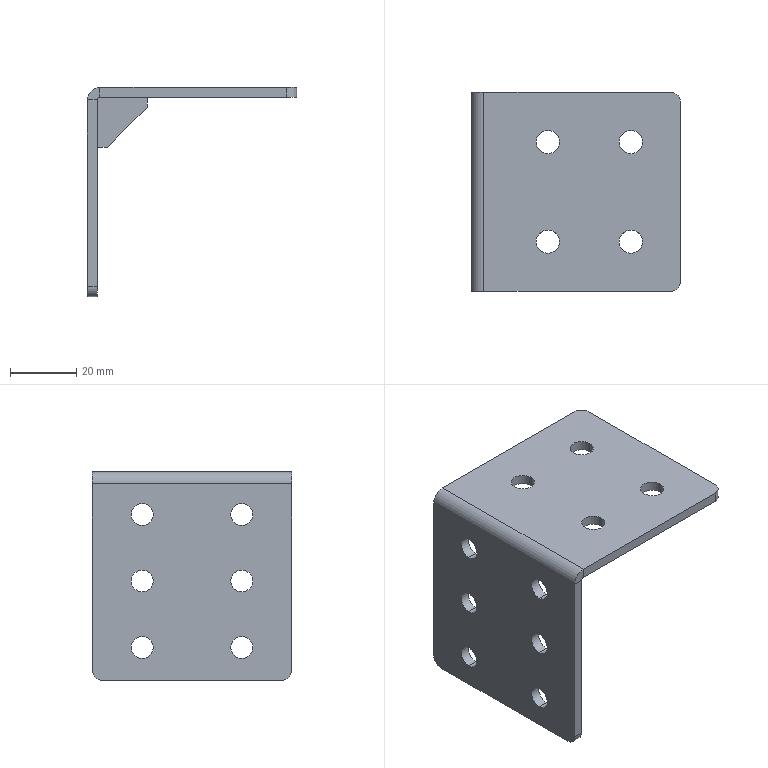Part | SolidWorks | features HoleWzd 2, Fillet 1, FlatPattern 1, ICE 1, SMBaseFlange 1, SheetMetal 1 | 1 solid | 44 faces | box 63 x 60 x 63 mm | volume 21324 mm3 | cylinder 27 | plane 17 | commonest cylinder face diameters 6.6 x12 7 x8 6 x4 1.5 x2 7.5 x1
STEP:
#1=CARTESIAN_POINT('',(23.5,45.,3.));
#2=VERTEX_POINT('',#1);
#3=CARTESIAN_POINT('',(16.5,45.,3.));
#4=VERTEX_POINT('',#3);
#5=CARTESIAN_POINT('',(20.,45.,3.));
#6=DIRECTION('',(0.,0.,-1.));
#7=DIRECTION('',(-1.,0.,0.));
#8=AXIS2_PLACEMENT_3D('',#5,#6,#7);
#9=CIRCLE('',#8,3.5);
#10=EDGE_CURVE('',#2,#4,#9,.T.);
#11=ORIENTED_EDGE('',*,*,#10,.F.);
#12=CARTESIAN_POINT('',(23.5,45.,0.));
#13=VERTEX_POINT('',#12);
#14=CARTESIAN_POINT('',(23.5,45.,0.));
#15=DIRECTION('',(0.,0.,-1.));
#16=VECTOR('',#15,1000.);
#17=LINE('',#14,#16);
#18=EDGE_CURVE('',#2,#13,#17,.T.);
#19=ORIENTED_EDGE('',*,*,#18,.T.);
#20=CARTESIAN_POINT('',(16.5,45.,0.));
#21=VERTEX_POINT('',#20);
#22=CARTESIAN_POINT('',(20.,45.,0.));
#23=DIRECTION('',(0.,0.,-1.));
#24=DIRECTION('',(-1.,0.,0.));
#25=AXIS2_PLACEMENT_3D('',#22,#23,#24);
#26=CIRCLE('',#25,3.5);
#27=EDGE_CURVE('',#13,#21,#26,.T.);
#28=ORIENTED_EDGE('',*,*,#27,.T.);
#29=CARTESIAN_POINT('',(16.5,45.,0.));
#30=DIRECTION('',(0.,0.,-1.));
#31=VECTOR('',#30,1000.);
#32=LINE('',#29,#31);
#33=EDGE_CURVE('',#4,#21,#32,.T.);
#34=ORIENTED_EDGE('',*,*,#33,.F.);
#35=EDGE_LOOP('',(#11,#19,#28,#34));
#36=FACE_OUTER_BOUND('',#35,.T.);
#37=CARTESIAN_POINT('',(20.,45.,0.));
#38=DIRECTION('',(0.,0.,-1.));
#39=DIRECTION('',(-1.,0.,0.));
#40=AXIS2_PLACEMENT_3D('',#37,#38,#39);
#41=CYLINDRICAL_SURFACE('',#40,3.5);
#42=ADVANCED_FACE('',(#36),#41,.F.);
#43=CARTESIAN_POINT('',(23.5,15.,3.));
#44=VERTEX_POINT('',#43);
#45=CARTESIAN_POINT('',(16.5,15.,3.));
#46=VERTEX_POINT('',#45);
#47=CARTESIAN_POINT('',(20.,15.,3.));
#48=DIRECTION('',(0.,0.,-1.));
#49=DIRECTION('',(-1.,0.,0.));
#50=AXIS2_PLACEMENT_3D('',#47,#48,#49);
#51=CIRCLE('',#50,3.5);
#52=EDGE_CURVE('',#44,#46,#51,.T.);
#53=ORIENTED_EDGE('',*,*,#52,.F.);
#54=CARTESIAN_POINT('',(23.5,15.,0.));
#55=VERTEX_POINT('',#54);
#56=CARTESIAN_POINT('',(23.5,15.,0.));
#57=DIRECTION('',(0.,0.,-1.));
#58=VECTOR('',#57,1000.);
#59=LINE('',#56,#58);
#60=EDGE_CURVE('',#44,#55,#59,.T.);
#61=ORIENTED_EDGE('',*,*,#60,.T.);
#62=CARTESIAN_POINT('',(16.5,15.,0.));
#63=VERTEX_POINT('',#62);
#64=CARTESIAN_POINT('',(20.,15.,0.));
#65=DIRECTION('',(0.,0.,-1.));
#66=DIRECTION('',(-1.,0.,0.));
#67=AXIS2_PLACEMENT_3D('',#64,#65,#66);
#68=CIRCLE('',#67,3.5);
#69=EDGE_CURVE('',#55,#63,#68,.T.);
#70=ORIENTED_EDGE('',*,*,#69,.T.);
#71=CARTESIAN_POINT('',(16.5,15.,0.));
#72=DIRECTION('',(0.,0.,-1.));
#73=VECTOR('',#72,1000.);
#74=LINE('',#71,#73);
#75=EDGE_CURVE('',#46,#63,#74,.T.);
#76=ORIENTED_EDGE('',*,*,#75,.F.);
#77=EDGE_LOOP('',(#53,#61,#70,#76));
#78=FACE_OUTER_BOUND('',#77,.T.);
#79=CARTESIAN_POINT('',(20.,15.,0.));
#80=DIRECTION('',(0.,0.,-1.));
#81=DIRECTION('',(-1.,0.,0.));
#82=AXIS2_PLACEMENT_3D('',#79,#80,#81);
#83=CYLINDRICAL_SURFACE('',#82,3.5);
#84=ADVANCED_FACE('',(#78),#83,.F.);
#85=CARTESIAN_POINT('',(48.5,45.,3.));
#86=VERTEX_POINT('',#85);
#87=CARTESIAN_POINT('',(41.5,45.,3.));
#88=VERTEX_POINT('',#87);
#89=CARTESIAN_POINT('',(45.,45.,3.));
#90=DIRECTION('',(0.,0.,-1.));
#91=DIRECTION('',(-1.,0.,0.));
#92=AXIS2_PLACEMENT_3D('',#89,#90,#91);
#93=CIRCLE('',#92,3.5);
#94=EDGE_CURVE('',#86,#88,#93,.T.);
#95=ORIENTED_EDGE('',*,*,#94,.F.);
#96=CARTESIAN_POINT('',(48.5,45.,0.));
#97=VERTEX_POINT('',#96);
#98=CARTESIAN_POINT('',(48.5,45.,0.));
#99=DIRECTION('',(0.,0.,-1.));
#100=VECTOR('',#99,1000.);
#101=LINE('',#98,#100);
#102=EDGE_CURVE('',#86,#97,#101,.T.);
#103=ORIENTED_EDGE('',*,*,#102,.T.);
#104=CARTESIAN_POINT('',(41.5,45.,0.));
#105=VERTEX_POINT('',#104);
#106=CARTESIAN_POINT('',(45.,45.,0.));
#107=DIRECTION('',(0.,0.,-1.));
#108=DIRECTION('',(-1.,0.,0.));
#109=AXIS2_PLACEMENT_3D('',#106,#107,#108);
#110=CIRCLE('',#109,3.5);
#111=EDGE_CURVE('',#97,#105,#110,.T.);
#112=ORIENTED_EDGE('',*,*,#111,.T.);
#113=CARTESIAN_POINT('',(41.5,45.,0.));
#114=DIRECTION('',(0.,0.,-1.));
#115=VECTOR('',#114,1000.);
#116=LINE('',#113,#115);
#117=EDGE_CURVE('',#88,#105,#116,.T.);
#118=ORIENTED_EDGE('',*,*,#117,.F.);
#119=EDGE_LOOP('',(#95,#103,#112,#118));
#120=FACE_OUTER_BOUND('',#119,.T.);
#121=CARTESIAN_POINT('',(45.,45.,0.));
#122=DIRECTION('',(0.,0.,-1.));
#123=DIRECTION('',(-1.,0.,0.));
#124=AXIS2_PLACEMENT_3D('',#121,#122,#123);
#125=CYLINDRICAL_SURFACE('',#124,3.5);
#126=ADVANCED_FACE('',(#120),#125,.F.);
#127=CARTESIAN_POINT('',(48.5,15.,3.));
#128=VERTEX_POINT('',#127);
#129=CARTESIAN_POINT('',(41.5,15.,3.));
#130=VERTEX_POINT('',#129);
#131=CARTESIAN_POINT('',(45.,15.,3.));
#132=DIRECTION('',(0.,0.,-1.));
#133=DIRECTION('',(-1.,0.,0.));
#134=AXIS2_PLACEMENT_3D('',#131,#132,#133);
#135=CIRCLE('',#134,3.5);
#136=EDGE_CURVE('',#128,#130,#135,.T.);
#137=ORIENTED_EDGE('',*,*,#136,.F.);
#138=CARTESIAN_POINT('',(48.5,15.,0.));
#139=VERTEX_POINT('',#138);
#140=CARTESIAN_POINT('',(48.5,15.,0.));
#141=DIRECTION('',(0.,0.,-1.));
#142=VECTOR('',#141,1000.);
#143=LINE('',#140,#142);
#144=EDGE_CURVE('',#128,#139,#143,.T.);
#145=ORIENTED_EDGE('',*,*,#144,.T.);
#146=CARTESIAN_POINT('',(41.5,15.,0.));
#147=VERTEX_POINT('',#146);
#148=CARTESIAN_POINT('',(45.,15.,0.));
#149=DIRECTION('',(0.,0.,-1.));
#150=DIRECTION('',(-1.,0.,0.));
#151=AXIS2_PLACEMENT_3D('',#148,#149,#150);
#152=CIRCLE('',#151,3.5);
#153=EDGE_CURVE('',#139,#147,#152,.T.);
#154=ORIENTED_EDGE('',*,*,#153,.T.);
#155=CARTESIAN_POINT('',(41.5,15.,0.));
#156=DIRECTION('',(0.,0.,-1.));
#157=VECTOR('',#156,1000.);
#158=LINE('',#155,#157);
#159=EDGE_CURVE('',#130,#147,#158,.T.);
#160=ORIENTED_EDGE('',*,*,#159,.F.);
#161=EDGE_LOOP('',(#137,#145,#154,#160));
#162=FACE_OUTER_BOUND('',#161,.T.);
#163=CARTESIAN_POINT('',(45.,15.,0.));
#164=DIRECTION('',(0.,0.,-1.));
#165=DIRECTION('',(-1.,0.,0.));
#166=AXIS2_PLACEMENT_3D('',#163,#164,#165);
#167=CYLINDRICAL_SURFACE('',#166,3.5);
#168=ADVANCED_FACE('',(#162),#167,.F.);
#169=CARTESIAN_POINT('',(-3.,45.,-46.7));
#170=VERTEX_POINT('',#169);
#171=CARTESIAN_POINT('',(-3.,45.,-53.3));
#172=VERTEX_POINT('',#171);
#173=CARTESIAN_POINT('',(-3.,45.,-50.));
#174=DIRECTION('',(1.,0.,0.));
#175=DIRECTION('',(0.,0.,-1.));
#176=AXIS2_PLACEMENT_3D('',#173,#174,#175);
#177=CIRCLE('',#176,3.3);
#178=EDGE_CURVE('',#170,#172,#177,.T.);
#179=ORIENTED_EDGE('',*,*,#178,.F.);
#180=CARTESIAN_POINT('',(0.,45.,-46.7));
#181=VERTEX_POINT('',#180);
#182=CARTESIAN_POINT('',(0.,45.,-46.7));
#183=DIRECTION('',(1.,0.,0.));
#184=VECTOR('',#183,1000.);
#185=LINE('',#182,#184);
#186=EDGE_CURVE('',#170,#181,#185,.T.);
#187=ORIENTED_EDGE('',*,*,#186,.T.);
#188=CARTESIAN_POINT('',(0.,45.,-53.3));
#189=VERTEX_POINT('',#188);
#190=CARTESIAN_POINT('',(0.,45.,-50.));
#191=DIRECTION('',(1.,0.,0.));
#192=DIRECTION('',(0.,0.,-1.));
#193=AXIS2_PLACEMENT_3D('',#190,#191,#192);
#194=CIRCLE('',#193,3.3);
#195=EDGE_CURVE('',#181,#189,#194,.T.);
#196=ORIENTED_EDGE('',*,*,#195,.T.);
#197=CARTESIAN_POINT('',(0.,45.,-53.3));
#198=DIRECTION('',(1.,0.,0.));
#199=VECTOR('',#198,1000.);
#200=LINE('',#197,#199);
#201=EDGE_CURVE('',#172,#189,#200,.T.);
#202=ORIENTED_EDGE('',*,*,#201,.F.);
#203=EDGE_LOOP('',(#179,#187,#196,#202));
#204=FACE_OUTER_BOUND('',#203,.T.);
#205=CARTESIAN_POINT('',(0.,45.,-50.));
#206=DIRECTION('',(1.,0.,0.));
#207=DIRECTION('',(0.,0.,-1.));
#208=AXIS2_PLACEMENT_3D('',#205,#206,#207);
#209=CYLINDRICAL_SURFACE('',#208,3.3);
#210=ADVANCED_FACE('',(#204),#209,.F.);
#211=CARTESIAN_POINT('',(-3.,45.,-26.7));
#212=VERTEX_POINT('',#211);
#213=CARTESIAN_POINT('',(-3.,45.,-33.3));
#214=VERTEX_POINT('',#213);
#215=CARTESIAN_POINT('',(-3.,45.,-30.));
#216=DIRECTION('',(1.,0.,0.));
#217=DIRECTION('',(0.,0.,-1.));
#218=AXIS2_PLACEMENT_3D('',#215,#216,#217);
#219=CIRCLE('',#218,3.3);
#220=EDGE_CURVE('',#212,#214,#219,.T.);
#221=ORIENTED_EDGE('',*,*,#220,.F.);
#222=CARTESIAN_POINT('',(0.,45.,-26.7));
#223=VERTEX_POINT('',#222);
#224=CARTESIAN_POINT('',(0.,45.,-26.7));
#225=DIRECTION('',(1.,0.,0.));
#226=VECTOR('',#225,1000.);
#227=LINE('',#224,#226);
#228=EDGE_CURVE('',#212,#223,#227,.T.);
#229=ORIENTED_EDGE('',*,*,#228,.T.);
#230=CARTESIAN_POINT('',(0.,45.,-33.3));
#231=VERTEX_POINT('',#230);
#232=CARTESIAN_POINT('',(0.,45.,-30.));
#233=DIRECTION('',(1.,0.,0.));
#234=DIRECTION('',(0.,0.,-1.));
#235=AXIS2_PLACEMENT_3D('',#232,#233,#234);
#236=CIRCLE('',#235,3.3);
#237=EDGE_CURVE('',#223,#231,#236,.T.);
#238=ORIENTED_EDGE('',*,*,#237,.T.);
#239=CARTESIAN_POINT('',(0.,45.,-33.3));
#240=DIRECTION('',(1.,0.,0.));
#241=VECTOR('',#240,1000.);
#242=LINE('',#239,#241);
#243=EDGE_CURVE('',#214,#231,#242,.T.);
#244=ORIENTED_EDGE('',*,*,#243,.F.);
#245=EDGE_LOOP('',(#221,#229,#238,#244));
#246=FACE_OUTER_BOUND('',#245,.T.);
#247=CARTESIAN_POINT('',(0.,45.,-30.));
#248=DIRECTION('',(1.,0.,0.));
#249=DIRECTION('',(0.,0.,-1.));
#250=AXIS2_PLACEMENT_3D('',#247,#248,#249);
#251=CYLINDRICAL_SURFACE('',#250,3.3);
#252=ADVANCED_FACE('',(#246),#251,.F.);
#253=CARTESIAN_POINT('',(-3.,45.,-6.7));
#254=VERTEX_POINT('',#253);
#255=CARTESIAN_POINT('',(-3.,45.,-13.3));
#256=VERTEX_POINT('',#255);
#257=CARTESIAN_POINT('',(-3.,45.,-10.));
#258=DIRECTION('',(1.,0.,0.));
#259=DIRECTION('',(0.,0.,-1.));
#260=AXIS2_PLACEMENT_3D('',#257,#258,#259);
#261=CIRCLE('',#260,3.3);
#262=EDGE_CURVE('',#254,#256,#261,.T.);
#263=ORIENTED_EDGE('',*,*,#262,.F.);
#264=CARTESIAN_POINT('',(0.,45.,-6.7));
#265=VERTEX_POINT('',#264);
#266=CARTESIAN_POINT('',(0.,45.,-6.7));
#267=DIRECTION('',(1.,0.,0.));
#268=VECTOR('',#267,1000.);
#269=LINE('',#266,#268);
#270=EDGE_CURVE('',#254,#265,#269,.T.);
#271=ORIENTED_EDGE('',*,*,#270,.T.);
#272=CARTESIAN_POINT('',(0.,45.,-13.3));
#273=VERTEX_POINT('',#272);
#274=CARTESIAN_POINT('',(0.,45.,-10.));
#275=DIRECTION('',(1.,0.,0.));
#276=DIRECTION('',(0.,0.,-1.));
#277=AXIS2_PLACEMENT_3D('',#274,#275,#276);
#278=CIRCLE('',#277,3.3);
#279=EDGE_CURVE('',#265,#273,#278,.T.);
#280=ORIENTED_EDGE('',*,*,#279,.T.);
#281=CARTESIAN_POINT('',(0.,45.,-13.3));
#282=DIRECTION('',(1.,0.,0.));
#283=VECTOR('',#282,1000.);
#284=LINE('',#281,#283);
#285=EDGE_CURVE('',#256,#273,#284,.T.);
#286=ORIENTED_EDGE('',*,*,#285,.F.);
#287=EDGE_LOOP('',(#263,#271,#280,#286));
#288=FACE_OUTER_BOUND('',#287,.T.);
#289=CARTESIAN_POINT('',(0.,45.,-10.));
#290=DIRECTION('',(1.,0.,0.));
#291=DIRECTION('',(0.,0.,-1.));
#292=AXIS2_PLACEMENT_3D('',#289,#290,#291);
#293=CYLINDRICAL_SURFACE('',#292,3.3);
#294=ADVANCED_FACE('',(#288),#293,.F.);
#295=CARTESIAN_POINT('',(-3.,15.,-46.7));
#296=VERTEX_POINT('',#295);
#297=CARTESIAN_POINT('',(-3.,15.,-53.3));
#298=VERTEX_POINT('',#297);
#299=CARTESIAN_POINT('',(-3.,15.,-50.));
#300=DIRECTION('',(1.,0.,0.));
#301=DIRECTION('',(0.,0.,-1.));
#302=AXIS2_PLACEMENT_3D('',#299,#300,#301);
#303=CIRCLE('',#302,3.3);
#304=EDGE_CURVE('',#296,#298,#303,.T.);
#305=ORIENTED_EDGE('',*,*,#304,.F.);
#306=CARTESIAN_POINT('',(0.,15.,-46.7));
#307=VERTEX_POINT('',#306);
#308=CARTESIAN_POINT('',(0.,15.,-46.7));
#309=DIRECTION('',(1.,0.,0.));
#310=VECTOR('',#309,1000.);
#311=LINE('',#308,#310);
#312=EDGE_CURVE('',#296,#307,#311,.T.);
#313=ORIENTED_EDGE('',*,*,#312,.T.);
#314=CARTESIAN_POINT('',(0.,15.,-53.3));
#315=VERTEX_POINT('',#314);
#316=CARTESIAN_POINT('',(0.,15.,-50.));
#317=DIRECTION('',(1.,0.,0.));
#318=DIRECTION('',(0.,0.,-1.));
#319=AXIS2_PLACEMENT_3D('',#316,#317,#318);
#320=CIRCLE('',#319,3.3);
#321=EDGE_CURVE('',#307,#315,#320,.T.);
#322=ORIENTED_EDGE('',*,*,#321,.T.);
#323=CARTESIAN_POINT('',(0.,15.,-53.3));
#324=DIRECTION('',(1.,0.,0.));
#325=VECTOR('',#324,1000.);
#326=LINE('',#323,#325);
#327=EDGE_CURVE('',#298,#315,#326,.T.);
#328=ORIENTED_EDGE('',*,*,#327,.F.);
#329=EDGE_LOOP('',(#305,#313,#322,#328));
#330=FACE_OUTER_BOUND('',#329,.T.);
#331=CARTESIAN_POINT('',(0.,15.,-50.));
#332=DIRECTION('',(1.,0.,0.));
#333=DIRECTION('',(0.,0.,-1.));
#334=AXIS2_PLACEMENT_3D('',#331,#332,#333);
#335=CYLINDRICAL_SURFACE('',#334,3.3);
#336=ADVANCED_FACE('',(#330),#335,.F.);
#337=CARTESIAN_POINT('',(-3.,15.,-26.7));
#338=VERTEX_POINT('',#337);
#339=CARTESIAN_POINT('',(-3.,15.,-33.3));
#340=VERTEX_POINT('',#339);
#341=CARTESIAN_POINT('',(-3.,15.,-30.));
#342=DIRECTION('',(1.,0.,0.));
#343=DIRECTION('',(0.,0.,-1.));
#344=AXIS2_PLACEMENT_3D('',#341,#342,#343);
#345=CIRCLE('',#344,3.3);
#346=EDGE_CURVE('',#338,#340,#345,.T.);
#347=ORIENTED_EDGE('',*,*,#346,.F.);
#348=CARTESIAN_POINT('',(0.,15.,-26.7));
#349=VERTEX_POINT('',#348);
#350=CARTESIAN_POINT('',(0.,15.,-26.7));
#351=DIRECTION('',(1.,0.,0.));
#352=VECTOR('',#351,1000.);
#353=LINE('',#350,#352);
#354=EDGE_CURVE('',#338,#349,#353,.T.);
#355=ORIENTED_EDGE('',*,*,#354,.T.);
#356=CARTESIAN_POINT('',(0.,15.,-33.3));
#357=VERTEX_POINT('',#356);
#358=CARTESIAN_POINT('',(0.,15.,-30.));
#359=DIRECTION('',(1.,0.,0.));
#360=DIRECTION('',(0.,0.,-1.));
#361=AXIS2_PLACEMENT_3D('',#358,#359,#360);
#362=CIRCLE('',#361,3.3);
#363=EDGE_CURVE('',#349,#357,#362,.T.);
#364=ORIENTED_EDGE('',*,*,#363,.T.);
#365=CARTESIAN_POINT('',(0.,15.,-33.3));
#366=DIRECTION('',(1.,0.,0.));
#367=VECTOR('',#366,1000.);
#368=LINE('',#365,#367);
#369=EDGE_CURVE('',#340,#357,#368,.T.);
#370=ORIENTED_EDGE('',*,*,#369,.F.);
#371=EDGE_LOOP('',(#347,#355,#364,#370));
#372=FACE_OUTER_BOUND('',#371,.T.);
#373=CARTESIAN_POINT('',(0.,15.,-30.));
#374=DIRECTION('',(1.,0.,0.));
#375=DIRECTION('',(0.,0.,-1.));
#376=AXIS2_PLACEMENT_3D('',#373,#374,#375);
#377=CYLINDRICAL_SURFACE('',#376,3.3);
#378=ADVANCED_FACE('',(#372),#377,.F.);
#379=CARTESIAN_POINT('',(-3.,15.,-6.7));
#380=VERTEX_POINT('',#379);
#381=CARTESIAN_POINT('',(-3.,15.,-13.3));
#382=VERTEX_POINT('',#381);
#383=CARTESIAN_POINT('',(-3.,15.,-10.));
#384=DIRECTION('',(1.,0.,0.));
#385=DIRECTION('',(0.,0.,-1.));
#386=AXIS2_PLACEMENT_3D('',#383,#384,#385);
#387=CIRCLE('',#386,3.3);
#388=EDGE_CURVE('',#380,#382,#387,.T.);
#389=ORIENTED_EDGE('',*,*,#388,.F.);
#390=CARTESIAN_POINT('',(0.,15.,-6.7));
#391=VERTEX_POINT('',#390);
#392=CARTESIAN_POINT('',(0.,15.,-6.7));
#393=DIRECTION('',(1.,0.,0.));
#394=VECTOR('',#393,1000.);
#395=LINE('',#392,#394);
#396=EDGE_CURVE('',#380,#391,#395,.T.);
#397=ORIENTED_EDGE('',*,*,#396,.T.);
#398=CARTESIAN_POINT('',(0.,15.,-13.3));
#399=VERTEX_POINT('',#398);
#400=CARTESIAN_POINT('',(0.,15.,-10.));
#401=DIRECTION('',(1.,0.,0.));
#402=DIRECTION('',(0.,0.,-1.));
#403=AXIS2_PLACEMENT_3D('',#400,#401,#402);
#404=CIRCLE('',#403,3.3);
#405=EDGE_CURVE('',#391,#399,#404,.T.);
#406=ORIENTED_EDGE('',*,*,#405,.T.);
#407=CARTESIAN_POINT('',(0.,15.,-13.3));
#408=DIRECTION('',(1.,0.,0.));
#409=VECTOR('',#408,1000.);
#410=LINE('',#407,#409);
#411=EDGE_CURVE('',#382,#399,#410,.T.);
#412=ORIENTED_EDGE('',*,*,#411,.F.);
#413=EDGE_LOOP('',(#389,#397,#406,#412));
#414=FACE_OUTER_BOUND('',#413,.T.);
#415=CARTESIAN_POINT('',(0.,15.,-10.));
#416=DIRECTION('',(1.,0.,0.));
#417=DIRECTION('',(0.,0.,-1.));
#418=AXIS2_PLACEMENT_3D('',#415,#416,#417);
#419=CYLINDRICAL_SURFACE('',#418,3.3);
#420=ADVANCED_FACE('',(#414),#419,.F.);
#421=CARTESIAN_POINT('',(0.,28.5,-0.75));
#422=VERTEX_POINT('',#421);
#423=CARTESIAN_POINT('',(0.,0.,-0.75));
#424=VERTEX_POINT('',#423);
#425=CARTESIAN_POINT('',(0.,60.,-0.75));
#426=DIRECTION('',(0.,-1.,0.));
#427=VECTOR('',#426,1000.);
#428=LINE('',#425,#427);
#429=EDGE_CURVE('',#422,#424,#428,.T.);
#430=ORIENTED_EDGE('',*,*,#429,.F.);
#431=CARTESIAN_POINT('',(0.75,28.5,0.));
#432=VERTEX_POINT('',#431);
#433=CARTESIAN_POINT('',(0.75,28.5,-0.75));
#434=DIRECTION('',(0.,1.,0.));
#435=DIRECTION('',(0.,0.,1.));
#436=AXIS2_PLACEMENT_3D('',#433,#434,#435);
#437=CIRCLE('',#436,0.75);
#438=EDGE_CURVE('',#422,#432,#437,.T.);
#439=ORIENTED_EDGE('',*,*,#438,.T.);
#440=CARTESIAN_POINT('',(0.75,0.,0.));
#441=VERTEX_POINT('',#440);
#442=CARTESIAN_POINT('',(0.75,60.,0.));
#443=DIRECTION('',(0.,-1.,0.));
#444=VECTOR('',#443,1000.);
#445=LINE('',#442,#444);
#446=EDGE_CURVE('',#432,#441,#445,.T.);
#447=ORIENTED_EDGE('',*,*,#446,.T.);
#448=CARTESIAN_POINT('',(0.75,0.,-0.75));
#449=DIRECTION('',(0.,1.,0.));
#450=DIRECTION('',(0.,0.,-1.));
#451=AXIS2_PLACEMENT_3D('',#448,#449,#450);
#452=CIRCLE('',#451,0.75);
#453=EDGE_CURVE('',#424,#441,#452,.T.);
#454=ORIENTED_EDGE('',*,*,#453,.F.);
#455=EDGE_LOOP('',(#430,#439,#447,#454));
#456=FACE_OUTER_BOUND('',#455,.T.);
#457=CARTESIAN_POINT('',(0.75,60.,-0.75));
#458=DIRECTION('',(0.,-1.,0.));
#459=DIRECTION('',(0.,0.,-1.));
#460=AXIS2_PLACEMENT_3D('',#457,#458,#459);
#461=CYLINDRICAL_SURFACE('',#460,0.75);
#462=ADVANCED_FACE('',(#456),#461,.F.);
#463=CARTESIAN_POINT('',(0.75,60.,0.));
#464=VERTEX_POINT('',#463);
#465=CARTESIAN_POINT('',(0.75,60.,3.));
#466=VERTEX_POINT('',#465);
#467=CARTESIAN_POINT('',(0.75,60.,0.));
#468=DIRECTION('',(0.,0.,1.));
#469=VECTOR('',#468,1000.);
#470=LINE('',#467,#469);
#471=EDGE_CURVE('',#464,#466,#470,.T.);
#472=ORIENTED_EDGE('',*,*,#471,.F.);
#473=CARTESIAN_POINT('',(0.,60.,-0.75));
#474=VERTEX_POINT('',#473);
#475=CARTESIAN_POINT('',(0.75,60.,-0.75));
#476=DIRECTION('',(0.,1.,0.));
#477=DIRECTION('',(0.,0.,-1.));
#478=AXIS2_PLACEMENT_3D('',#475,#476,#477);
#479=CIRCLE('',#478,0.75);
#480=EDGE_CURVE('',#474,#464,#479,.T.);
#481=ORIENTED_EDGE('',*,*,#480,.F.);
#482=CARTESIAN_POINT('',(-3.,60.,-0.75));
#483=VERTEX_POINT('',#482);
#484=CARTESIAN_POINT('',(-3.,60.,-0.75));
#485=DIRECTION('',(1.,0.,0.));
#486=VECTOR('',#485,1000.);
#487=LINE('',#484,#486);
#488=EDGE_CURVE('',#483,#474,#487,.T.);
#489=ORIENTED_EDGE('',*,*,#488,.F.);
#490=CARTESIAN_POINT('',(0.75,60.,-0.75));
#491=DIRECTION('',(0.,1.,0.));
#492=DIRECTION('',(1.,0.,0.));
#493=AXIS2_PLACEMENT_3D('',#490,#491,#492);
#494=CIRCLE('',#493,3.75);
#495=EDGE_CURVE('',#483,#466,#494,.T.);
#496=ORIENTED_EDGE('',*,*,#495,.T.);
#497=EDGE_LOOP('',(#472,#481,#489,#496));
#498=FACE_OUTER_BOUND('',#497,.T.);
#499=CARTESIAN_POINT('',(0.75,60.,0.));
#500=DIRECTION('',(0.,1.,0.));
#501=DIRECTION('',(0.,0.,1.));
#502=AXIS2_PLACEMENT_3D('',#499,#500,#501);
#503=PLANE('',#502);
#504=ADVANCED_FACE('',(#498),#503,.T.);
#505=CARTESIAN_POINT('',(57.,60.,3.));
#506=VERTEX_POINT('',#505);
#507=CARTESIAN_POINT('',(0.,60.,3.));
#508=DIRECTION('',(1.,0.,0.));
#509=VECTOR('',#508,1000.);
#510=LINE('',#507,#509);
#511=EDGE_CURVE('',#466,#506,#510,.T.);
#512=ORIENTED_EDGE('',*,*,#511,.T.);
#513=CARTESIAN_POINT('',(57.,60.,0.));
#514=VERTEX_POINT('',#513);
#515=CARTESIAN_POINT('',(57.,60.,-0.75));
#516=DIRECTION('',(0.,0.,-1.));
#517=VECTOR('',#516,1000.);
#518=LINE('',#515,#517);
#519=EDGE_CURVE('',#506,#514,#518,.T.);
#520=ORIENTED_EDGE('',*,*,#519,.T.);
#521=CARTESIAN_POINT('',(0.,60.,0.));
#522=DIRECTION('',(1.,0.,0.));
#523=VECTOR('',#522,1000.);
#524=LINE('',#521,#523);
#525=EDGE_CURVE('',#464,#514,#524,.T.);
#526=ORIENTED_EDGE('',*,*,#525,.F.);
#527=ORIENTED_EDGE('',*,*,#471,.T.);
#528=EDGE_LOOP('',(#512,#520,#526,#527));
#529=FACE_OUTER_BOUND('',#528,.T.);
#530=CARTESIAN_POINT('',(-3.,60.,-0.75));
#531=DIRECTION('',(0.,1.,0.));
#532=DIRECTION('',(0.,0.,1.));
#533=AXIS2_PLACEMENT_3D('',#530,#531,#532);
#534=PLANE('',#533);
#535=ADVANCED_FACE('',(#529),#534,.T.);
#536=CARTESIAN_POINT('',(-3.,0.,-0.75));
#537=VERTEX_POINT('',#536);
#538=CARTESIAN_POINT('',(0.,0.,-0.75));
#539=DIRECTION('',(-1.,0.,0.));
#540=VECTOR('',#539,1000.);
#541=LINE('',#538,#540);
#542=EDGE_CURVE('',#424,#537,#541,.T.);
#543=ORIENTED_EDGE('',*,*,#542,.F.);
#544=ORIENTED_EDGE('',*,*,#453,.T.);
#545=CARTESIAN_POINT('',(0.75,0.,3.));
#546=VERTEX_POINT('',#545);
#547=CARTESIAN_POINT('',(0.75,0.,3.));
#548=DIRECTION('',(0.,0.,-1.));
#549=VECTOR('',#548,1000.);
#550=LINE('',#547,#549);
#551=EDGE_CURVE('',#546,#441,#550,.T.);
#552=ORIENTED_EDGE('',*,*,#551,.F.);
#553=CARTESIAN_POINT('',(0.75,0.,-0.75));
#554=DIRECTION('',(0.,1.,0.));
#555=DIRECTION('',(1.,0.,0.));
#556=AXIS2_PLACEMENT_3D('',#553,#554,#555);
#557=CIRCLE('',#556,3.75);
#558=EDGE_CURVE('',#537,#546,#557,.T.);
#559=ORIENTED_EDGE('',*,*,#558,.F.);
#560=EDGE_LOOP('',(#543,#544,#552,#559));
#561=FACE_OUTER_BOUND('',#560,.T.);
#562=CARTESIAN_POINT('',(0.,0.,-0.75));
#563=DIRECTION('',(0.,-1.,0.));
#564=DIRECTION('',(0.,0.,-1.));
#565=AXIS2_PLACEMENT_3D('',#562,#563,#564);
#566=PLANE('',#565);
#567=ADVANCED_FACE('',(#561),#566,.T.);
#568=CARTESIAN_POINT('',(-3.,0.,-57.));
#569=VERTEX_POINT('',#568);
#570=CARTESIAN_POINT('',(-3.,0.,-60.));
#571=DIRECTION('',(0.,0.,1.));
#572=VECTOR('',#571,1000.);
#573=LINE('',#570,#572);
#574=EDGE_CURVE('',#569,#537,#573,.T.);
#575=ORIENTED_EDGE('',*,*,#574,.F.);
#576=CARTESIAN_POINT('',(0.,0.,-57.));
#577=VERTEX_POINT('',#576);
#578=CARTESIAN_POINT('',(0.75,0.,-57.));
#579=DIRECTION('',(1.,0.,0.));
#580=VECTOR('',#579,1000.);
#581=LINE('',#578,#580);
#582=EDGE_CURVE('',#569,#577,#581,.T.);
#583=ORIENTED_EDGE('',*,*,#582,.T.);
#584=CARTESIAN_POINT('',(0.,0.,-60.));
#585=DIRECTION('',(0.,0.,1.));
#586=VECTOR('',#585,1000.);
#587=LINE('',#584,#586);
#588=EDGE_CURVE('',#577,#424,#587,.T.);
#589=ORIENTED_EDGE('',*,*,#588,.T.);
#590=ORIENTED_EDGE('',*,*,#542,.T.);
#591=EDGE_LOOP('',(#575,#583,#589,#590));
#592=FACE_OUTER_BOUND('',#591,.T.);
#593=CARTESIAN_POINT('',(0.75,0.,3.));
#594=DIRECTION('',(0.,-1.,0.));
#595=DIRECTION('',(0.,0.,-1.));
#596=AXIS2_PLACEMENT_3D('',#593,#594,#595);
#597=PLANE('',#596);
#598=ADVANCED_FACE('',(#592),#597,.T.);
#599=CARTESIAN_POINT('',(20.,45.,3.));
#600=DIRECTION('',(0.,0.,-1.));
#601=DIRECTION('',(-1.,0.,0.));
#602=AXIS2_PLACEMENT_3D('',#599,#600,#601);
#603=CIRCLE('',#602,3.5);
#604=EDGE_CURVE('',#4,#2,#603,.T.);
#605=ORIENTED_EDGE('',*,*,#604,.T.);
#606=ORIENTED_EDGE('',*,*,#10,.T.);
#607=EDGE_LOOP('',(#605,#606));
#608=FACE_BOUND('',#607,.T.);
#609=CARTESIAN_POINT('',(20.,15.,3.));
#610=DIRECTION('',(0.,0.,-1.));
#611=DIRECTION('',(-1.,0.,0.));
#612=AXIS2_PLACEMENT_3D('',#609,#610,#611);
#613=CIRCLE('',#612,3.5);
#614=EDGE_CURVE('',#46,#44,#613,.T.);
#615=ORIENTED_EDGE('',*,*,#614,.T.);
#616=ORIENTED_EDGE('',*,*,#52,.T.);
#617=EDGE_LOOP('',(#615,#616));
#618=FACE_BOUND('',#617,.T.);
#619=CARTESIAN_POINT('',(45.,45.,3.));
#620=DIRECTION('',(0.,0.,-1.));
#621=DIRECTION('',(-1.,0.,0.));
#622=AXIS2_PLACEMENT_3D('',#619,#620,#621);
#623=CIRCLE('',#622,3.5);
#624=EDGE_CURVE('',#88,#86,#623,.T.);
#625=ORIENTED_EDGE('',*,*,#624,.T.);
#626=ORIENTED_EDGE('',*,*,#94,.T.);
#627=EDGE_LOOP('',(#625,#626));
#628=FACE_BOUND('',#627,.T.);
#629=CARTESIAN_POINT('',(45.,15.,3.));
#630=DIRECTION('',(0.,0.,-1.));
#631=DIRECTION('',(-1.,0.,0.));
#632=AXIS2_PLACEMENT_3D('',#629,#630,#631);
#633=CIRCLE('',#632,3.5);
#634=EDGE_CURVE('',#130,#128,#633,.T.);
#635=ORIENTED_EDGE('',*,*,#634,.T.);
#636=ORIENTED_EDGE('',*,*,#136,.T.);
#637=EDGE_LOOP('',(#635,#636));
#638=FACE_BOUND('',#637,.T.);
#639=CARTESIAN_POINT('',(57.,0.,3.));
#640=VERTEX_POINT('',#639);
#641=CARTESIAN_POINT('',(0.,0.,3.));
#642=DIRECTION('',(1.,0.,0.));
#643=VECTOR('',#642,1000.);
#644=LINE('',#641,#643);
#645=EDGE_CURVE('',#546,#640,#644,.T.);
#646=ORIENTED_EDGE('',*,*,#645,.T.);
#647=CARTESIAN_POINT('',(60.,3.,3.));
#648=VERTEX_POINT('',#647);
#649=CARTESIAN_POINT('',(57.,3.,3.));
#650=DIRECTION('',(0.,0.,1.));
#651=DIRECTION('',(-1.,0.,0.));
#652=AXIS2_PLACEMENT_3D('',#649,#650,#651);
#653=CIRCLE('',#652,3.);
#654=EDGE_CURVE('',#640,#648,#653,.T.);
#655=ORIENTED_EDGE('',*,*,#654,.T.);
#656=CARTESIAN_POINT('',(60.,57.,3.));
#657=VERTEX_POINT('',#656);
#658=CARTESIAN_POINT('',(60.,60.,3.));
#659=DIRECTION('',(0.,-1.,0.));
#660=VECTOR('',#659,1000.);
#661=LINE('',#658,#660);
#662=EDGE_CURVE('',#657,#648,#661,.T.);
#663=ORIENTED_EDGE('',*,*,#662,.F.);
#664=CARTESIAN_POINT('',(57.,57.,3.));
#665=DIRECTION('',(0.,0.,1.));
#666=DIRECTION('',(-1.,0.,0.));
#667=AXIS2_PLACEMENT_3D('',#664,#665,#666);
#668=CIRCLE('',#667,3.);
#669=EDGE_CURVE('',#657,#506,#668,.T.);
#670=ORIENTED_EDGE('',*,*,#669,.T.);
#671=ORIENTED_EDGE('',*,*,#511,.F.);
#672=CARTESIAN_POINT('',(0.75,60.,3.));
#673=DIRECTION('',(0.,-1.,0.));
#674=VECTOR('',#673,1000.);
#675=LINE('',#672,#674);
#676=EDGE_CURVE('',#466,#546,#675,.T.);
#677=ORIENTED_EDGE('',*,*,#676,.T.);
#678=EDGE_LOOP('',(#646,#655,#663,#670,#671,#677));
#679=FACE_OUTER_BOUND('',#678,.T.);
#680=CARTESIAN_POINT('',(0.,60.,3.));
#681=DIRECTION('',(0.,0.,-1.));
#682=DIRECTION('',(-1.,0.,0.));
#683=AXIS2_PLACEMENT_3D('',#680,#681,#682);
#684=PLANE('',#683);
#685=ADVANCED_FACE('',(#608,#618,#628,#638,#679),#684,.F.);
#686=ORIENTED_EDGE('',*,*,#662,.T.);
#687=CARTESIAN_POINT('',(60.,3.,0.));
#688=VERTEX_POINT('',#687);
#689=CARTESIAN_POINT('',(60.,3.,0.));
#690=DIRECTION('',(0.,0.,-1.));
#691=VECTOR('',#690,1000.);
#692=LINE('',#689,#691);
#693=EDGE_CURVE('',#648,#688,#692,.T.);
#694=ORIENTED_EDGE('',*,*,#693,.T.);
#695=CARTESIAN_POINT('',(60.,57.,0.));
#696=VERTEX_POINT('',#695);
#697=CARTESIAN_POINT('',(60.,60.,0.));
#698=DIRECTION('',(0.,-1.,0.));
#699=VECTOR('',#698,1000.);
#700=LINE('',#697,#699);
#701=EDGE_CURVE('',#696,#688,#700,.T.);
#702=ORIENTED_EDGE('',*,*,#701,.F.);
#703=CARTESIAN_POINT('',(60.,57.,0.));
#704=DIRECTION('',(0.,0.,1.));
#705=VECTOR('',#704,1000.);
#706=LINE('',#703,#705);
#707=EDGE_CURVE('',#696,#657,#706,.T.);
#708=ORIENTED_EDGE('',*,*,#707,.T.);
#709=EDGE_LOOP('',(#686,#694,#702,#708));
#710=FACE_OUTER_BOUND('',#709,.T.);
#711=CARTESIAN_POINT('',(60.,60.,0.));
#712=DIRECTION('',(1.,0.,0.));
#713=DIRECTION('',(0.,0.,-1.));
#714=AXIS2_PLACEMENT_3D('',#711,#712,#713);
#715=PLANE('',#714);
#716=ADVANCED_FACE('',(#710),#715,.T.);
#717=CARTESIAN_POINT('',(20.,45.,0.));
#718=DIRECTION('',(0.,0.,-1.));
#719=DIRECTION('',(-1.,0.,0.));
#720=AXIS2_PLACEMENT_3D('',#717,#718,#719);
#721=CIRCLE('',#720,3.5);
#722=EDGE_CURVE('',#21,#13,#721,.T.);
#723=ORIENTED_EDGE('',*,*,#722,.F.);
#724=ORIENTED_EDGE('',*,*,#27,.F.);
#725=EDGE_LOOP('',(#723,#724));
#726=FACE_BOUND('',#725,.T.);
#727=CARTESIAN_POINT('',(20.,15.,0.));
#728=DIRECTION('',(0.,0.,-1.));
#729=DIRECTION('',(-1.,0.,0.));
#730=AXIS2_PLACEMENT_3D('',#727,#728,#729);
#731=CIRCLE('',#730,3.5);
#732=EDGE_CURVE('',#63,#55,#731,.T.);
#733=ORIENTED_EDGE('',*,*,#732,.F.);
#734=ORIENTED_EDGE('',*,*,#69,.F.);
#735=EDGE_LOOP('',(#733,#734));
#736=FACE_BOUND('',#735,.T.);
#737=CARTESIAN_POINT('',(45.,45.,0.));
#738=DIRECTION('',(0.,0.,-1.));
#739=DIRECTION('',(-1.,0.,0.));
#740=AXIS2_PLACEMENT_3D('',#737,#738,#739);
#741=CIRCLE('',#740,3.5);
#742=EDGE_CURVE('',#105,#97,#741,.T.);
#743=ORIENTED_EDGE('',*,*,#742,.F.);
#744=ORIENTED_EDGE('',*,*,#111,.F.);
#745=EDGE_LOOP('',(#743,#744));
#746=FACE_BOUND('',#745,.T.);
#747=CARTESIAN_POINT('',(45.,15.,0.));
#748=DIRECTION('',(0.,0.,-1.));
#749=DIRECTION('',(-1.,0.,0.));
#750=AXIS2_PLACEMENT_3D('',#747,#748,#749);
#751=CIRCLE('',#750,3.5);
#752=EDGE_CURVE('',#147,#139,#751,.T.);
#753=ORIENTED_EDGE('',*,*,#752,.F.);
#754=ORIENTED_EDGE('',*,*,#153,.F.);
#755=EDGE_LOOP('',(#753,#754));
#756=FACE_BOUND('',#755,.T.);
#757=CARTESIAN_POINT('',(0.75,31.5,0.));
#758=VERTEX_POINT('',#757);
#759=CARTESIAN_POINT('',(15.,31.5,0.));
#760=VERTEX_POINT('',#759);
#761=CARTESIAN_POINT('',(0.75,31.5,0.));
#762=DIRECTION('',(1.,0.,0.));
#763=VECTOR('',#762,1000.);
#764=LINE('',#761,#763);
#765=EDGE_CURVE('',#758,#760,#764,.T.);
#766=ORIENTED_EDGE('',*,*,#765,.F.);
#767=CARTESIAN_POINT('',(0.75,60.,0.));
#768=DIRECTION('',(0.,-1.,0.));
#769=VECTOR('',#768,1000.);
#770=LINE('',#767,#769);
#771=EDGE_CURVE('',#464,#758,#770,.T.);
#772=ORIENTED_EDGE('',*,*,#771,.F.);
#773=ORIENTED_EDGE('',*,*,#525,.T.);
#774=CARTESIAN_POINT('',(57.,57.,0.));
#775=DIRECTION('',(0.,0.,-1.));
#776=DIRECTION('',(-1.,0.,0.));
#777=AXIS2_PLACEMENT_3D('',#774,#775,#776);
#778=CIRCLE('',#777,3.);
#779=EDGE_CURVE('',#514,#696,#778,.T.);
#780=ORIENTED_EDGE('',*,*,#779,.T.);
#781=ORIENTED_EDGE('',*,*,#701,.T.);
#782=CARTESIAN_POINT('',(57.,0.,0.));
#783=VERTEX_POINT('',#782);
#784=CARTESIAN_POINT('',(57.,3.,0.));
#785=DIRECTION('',(0.,0.,-1.));
#786=DIRECTION('',(-1.,0.,0.));
#787=AXIS2_PLACEMENT_3D('',#784,#785,#786);
#788=CIRCLE('',#787,3.);
#789=EDGE_CURVE('',#688,#783,#788,.T.);
#790=ORIENTED_EDGE('',*,*,#789,.T.);
#791=CARTESIAN_POINT('',(0.,0.,0.));
#792=DIRECTION('',(1.,0.,0.));
#793=VECTOR('',#792,1000.);
#794=LINE('',#791,#793);
#795=EDGE_CURVE('',#441,#783,#794,.T.);
#796=ORIENTED_EDGE('',*,*,#795,.F.);
#797=ORIENTED_EDGE('',*,*,#446,.F.);
#798=CARTESIAN_POINT('',(15.,28.5,0.));
#799=VERTEX_POINT('',#798);
#800=CARTESIAN_POINT('',(0.75,28.5,0.));
#801=DIRECTION('',(1.,0.,0.));
#802=VECTOR('',#801,1000.);
#803=LINE('',#800,#802);
#804=EDGE_CURVE('',#432,#799,#803,.T.);
#805=ORIENTED_EDGE('',*,*,#804,.T.);
#806=CARTESIAN_POINT('',(15.,31.5,0.));
#807=DIRECTION('',(0.,-1.,0.));
#808=VECTOR('',#807,1000.);
#809=LINE('',#806,#808);
#810=EDGE_CURVE('',#760,#799,#809,.T.);
#811=ORIENTED_EDGE('',*,*,#810,.F.);
#812=EDGE_LOOP('',(#766,#772,#773,#780,#781,#790,#796,#797,#805,#811));
#813=FACE_OUTER_BOUND('',#812,.T.);
#814=CARTESIAN_POINT('',(0.,60.,0.));
#815=DIRECTION('',(0.,0.,-1.));
#816=DIRECTION('',(-1.,0.,0.));
#817=AXIS2_PLACEMENT_3D('',#814,#815,#816);
#818=PLANE('',#817);
#819=ADVANCED_FACE('',(#726,#736,#746,#756,#813),#818,.T.);
#820=CARTESIAN_POINT('',(0.,31.5,-0.75));
#821=VERTEX_POINT('',#820);
#822=CARTESIAN_POINT('',(0.75,31.5,-0.75));
#823=DIRECTION('',(0.,1.,0.));
#824=DIRECTION('',(0.,0.,1.));
#825=AXIS2_PLACEMENT_3D('',#822,#823,#824);
#826=CIRCLE('',#825,0.75);
#827=EDGE_CURVE('',#821,#758,#826,.T.);
#828=ORIENTED_EDGE('',*,*,#827,.F.);
#829=CARTESIAN_POINT('',(0.,60.,-0.75));
#830=DIRECTION('',(0.,-1.,0.));
#831=VECTOR('',#830,1000.);
#832=LINE('',#829,#831);
#833=EDGE_CURVE('',#474,#821,#832,.T.);
#834=ORIENTED_EDGE('',*,*,#833,.F.);
#835=ORIENTED_EDGE('',*,*,#480,.T.);
#836=ORIENTED_EDGE('',*,*,#771,.T.);
#837=EDGE_LOOP('',(#828,#834,#835,#836));
#838=FACE_OUTER_BOUND('',#837,.T.);
#839=CARTESIAN_POINT('',(0.75,60.,-0.75));
#840=DIRECTION('',(0.,-1.,0.));
#841=DIRECTION('',(0.,0.,-1.));
#842=AXIS2_PLACEMENT_3D('',#839,#840,#841);
#843=CYLINDRICAL_SURFACE('',#842,0.75);
#844=ADVANCED_FACE('',(#838),#843,.F.);
#845=CARTESIAN_POINT('',(0.,45.,-50.));
#846=DIRECTION('',(1.,0.,0.));
#847=DIRECTION('',(0.,0.,-1.));
#848=AXIS2_PLACEMENT_3D('',#845,#846,#847);
#849=CIRCLE('',#848,3.3);
#850=EDGE_CURVE('',#189,#181,#849,.T.);
#851=ORIENTED_EDGE('',*,*,#850,.F.);
#852=ORIENTED_EDGE('',*,*,#195,.F.);
#853=EDGE_LOOP('',(#851,#852));
#854=FACE_BOUND('',#853,.T.);
#855=CARTESIAN_POINT('',(0.,45.,-30.));
#856=DIRECTION('',(1.,0.,0.));
#857=DIRECTION('',(0.,0.,-1.));
#858=AXIS2_PLACEMENT_3D('',#855,#856,#857);
#859=CIRCLE('',#858,3.3);
#860=EDGE_CURVE('',#231,#223,#859,.T.);
#861=ORIENTED_EDGE('',*,*,#860,.F.);
#862=ORIENTED_EDGE('',*,*,#237,.F.);
#863=EDGE_LOOP('',(#861,#862));
#864=FACE_BOUND('',#863,.T.);
#865=CARTESIAN_POINT('',(0.,45.,-10.));
#866=DIRECTION('',(1.,0.,0.));
#867=DIRECTION('',(0.,0.,-1.));
#868=AXIS2_PLACEMENT_3D('',#865,#866,#867);
#869=CIRCLE('',#868,3.3);
#870=EDGE_CURVE('',#273,#265,#869,.T.);
#871=ORIENTED_EDGE('',*,*,#870,.F.);
#872=ORIENTED_EDGE('',*,*,#279,.F.);
#873=EDGE_LOOP('',(#871,#872));
#874=FACE_BOUND('',#873,.T.);
#875=CARTESIAN_POINT('',(0.,15.,-50.));
#876=DIRECTION('',(1.,0.,0.));
#877=DIRECTION('',(0.,0.,-1.));
#878=AXIS2_PLACEMENT_3D('',#875,#876,#877);
#879=CIRCLE('',#878,3.3);
#880=EDGE_CURVE('',#315,#307,#879,.T.);
#881=ORIENTED_EDGE('',*,*,#880,.F.);
#882=ORIENTED_EDGE('',*,*,#321,.F.);
#883=EDGE_LOOP('',(#881,#882));
#884=FACE_BOUND('',#883,.T.);
#885=CARTESIAN_POINT('',(0.,15.,-30.));
#886=DIRECTION('',(1.,0.,0.));
#887=DIRECTION('',(0.,0.,-1.));
#888=AXIS2_PLACEMENT_3D('',#885,#886,#887);
#889=CIRCLE('',#888,3.3);
#890=EDGE_CURVE('',#357,#349,#889,.T.);
#891=ORIENTED_EDGE('',*,*,#890,.F.);
#892=ORIENTED_EDGE('',*,*,#363,.F.);
#893=EDGE_LOOP('',(#891,#892));
#894=FACE_BOUND('',#893,.T.);
#895=CARTESIAN_POINT('',(0.,15.,-10.));
#896=DIRECTION('',(1.,0.,0.));
#897=DIRECTION('',(0.,0.,-1.));
#898=AXIS2_PLACEMENT_3D('',#895,#896,#897);
#899=CIRCLE('',#898,3.3);
#900=EDGE_CURVE('',#399,#391,#899,.T.);
#901=ORIENTED_EDGE('',*,*,#900,.F.);
#902=ORIENTED_EDGE('',*,*,#405,.F.);
#903=EDGE_LOOP('',(#901,#902));
#904=FACE_BOUND('',#903,.T.);
#905=CARTESIAN_POINT('',(0.,31.5,-15.));
#906=VERTEX_POINT('',#905);
#907=CARTESIAN_POINT('',(0.,31.5,-15.));
#908=DIRECTION('',(0.,0.,1.));
#909=VECTOR('',#908,1000.);
#910=LINE('',#907,#909);
#911=EDGE_CURVE('',#906,#821,#910,.T.);
#912=ORIENTED_EDGE('',*,*,#911,.F.);
#913=CARTESIAN_POINT('',(0.,28.5,-15.));
#914=VERTEX_POINT('',#913);
#915=CARTESIAN_POINT('',(0.,31.5,-15.));
#916=DIRECTION('',(0.,-1.,0.));
#917=VECTOR('',#916,1000.);
#918=LINE('',#915,#917);
#919=EDGE_CURVE('',#906,#914,#918,.T.);
#920=ORIENTED_EDGE('',*,*,#919,.T.);
#921=CARTESIAN_POINT('',(0.,28.5,-15.));
#922=DIRECTION('',(0.,0.,1.));
#923=VECTOR('',#922,1000.);
#924=LINE('',#921,#923);
#925=EDGE_CURVE('',#914,#422,#924,.T.);
#926=ORIENTED_EDGE('',*,*,#925,.T.);
#927=ORIENTED_EDGE('',*,*,#429,.T.);
#928=ORIENTED_EDGE('',*,*,#588,.F.);
#929=CARTESIAN_POINT('',(0.,3.,-60.));
#930=VERTEX_POINT('',#929);
#931=CARTESIAN_POINT('',(0.,3.,-57.));
#932=DIRECTION('',(1.,0.,0.));
#933=DIRECTION('',(0.,0.,-1.));
#934=AXIS2_PLACEMENT_3D('',#931,#932,#933);
#935=CIRCLE('',#934,3.);
#936=EDGE_CURVE('',#577,#930,#935,.T.);
#937=ORIENTED_EDGE('',*,*,#936,.T.);
#938=CARTESIAN_POINT('',(0.,57.,-60.));
#939=VERTEX_POINT('',#938);
#940=CARTESIAN_POINT('',(0.,60.,-60.));
#941=DIRECTION('',(0.,-1.,0.));
#942=VECTOR('',#941,1000.);
#943=LINE('',#940,#942);
#944=EDGE_CURVE('',#939,#930,#943,.T.);
#945=ORIENTED_EDGE('',*,*,#944,.F.);
#946=CARTESIAN_POINT('',(0.,60.,-57.));
#947=VERTEX_POINT('',#946);
#948=CARTESIAN_POINT('',(0.,57.,-57.));
#949=DIRECTION('',(1.,0.,0.));
#950=DIRECTION('',(0.,0.,-1.));
#951=AXIS2_PLACEMENT_3D('',#948,#949,#950);
#952=CIRCLE('',#951,3.);
#953=EDGE_CURVE('',#939,#947,#952,.T.);
#954=ORIENTED_EDGE('',*,*,#953,.T.);
#955=CARTESIAN_POINT('',(0.,60.,-60.));
#956=DIRECTION('',(0.,0.,1.));
#957=VECTOR('',#956,1000.);
#958=LINE('',#955,#957);
#959=EDGE_CURVE('',#947,#474,#958,.T.);
#960=ORIENTED_EDGE('',*,*,#959,.T.);
#961=ORIENTED_EDGE('',*,*,#833,.T.);
#962=EDGE_LOOP('',(#912,#920,#926,#927,#928,#937,#945,#954,#960,#961));
#963=FACE_OUTER_BOUND('',#962,.T.);
#964=CARTESIAN_POINT('',(0.,60.,-60.));
#965=DIRECTION('',(1.,0.,0.));
#966=DIRECTION('',(0.,0.,-1.));
#967=AXIS2_PLACEMENT_3D('',#964,#965,#966);
#968=PLANE('',#967);
#969=ADVANCED_FACE('',(#854,#864,#874,#884,#894,#904,#963),#968,.T.);
#970=ORIENTED_EDGE('',*,*,#944,.T.);
#971=CARTESIAN_POINT('',(-3.,3.,-60.));
#972=VERTEX_POINT('',#971);
#973=CARTESIAN_POINT('',(-3.,3.,-60.));
#974=DIRECTION('',(-1.,0.,0.));
#975=VECTOR('',#974,1000.);
#976=LINE('',#973,#975);
#977=EDGE_CURVE('',#930,#972,#976,.T.);
#978=ORIENTED_EDGE('',*,*,#977,.T.);
#979=CARTESIAN_POINT('',(-3.,57.,-60.));
#980=VERTEX_POINT('',#979);
#981=CARTESIAN_POINT('',(-3.,60.,-60.));
#982=DIRECTION('',(0.,-1.,0.));
#983=VECTOR('',#982,1000.);
#984=LINE('',#981,#983);
#985=EDGE_CURVE('',#980,#972,#984,.T.);
#986=ORIENTED_EDGE('',*,*,#985,.F.);
#987=CARTESIAN_POINT('',(0.,57.,-60.));
#988=DIRECTION('',(1.,0.,0.));
#989=VECTOR('',#988,1000.);
#990=LINE('',#987,#989);
#991=EDGE_CURVE('',#980,#939,#990,.T.);
#992=ORIENTED_EDGE('',*,*,#991,.T.);
#993=EDGE_LOOP('',(#970,#978,#986,#992));
#994=FACE_OUTER_BOUND('',#993,.T.);
#995=CARTESIAN_POINT('',(-3.,60.,-60.));
#996=DIRECTION('',(0.,0.,-1.));
#997=DIRECTION('',(-1.,0.,0.));
#998=AXIS2_PLACEMENT_3D('',#995,#996,#997);
#999=PLANE('',#998);
#1000=ADVANCED_FACE('',(#994),#999,.T.);
#1001=CARTESIAN_POINT('',(-3.,45.,-50.));
#1002=DIRECTION('',(1.,0.,0.));
#1003=DIRECTION('',(0.,0.,-1.));
#1004=AXIS2_PLACEMENT_3D('',#1001,#1002,#1003);
#1005=CIRCLE('',#1004,3.3);
#1006=EDGE_CURVE('',#172,#170,#1005,.T.);
#1007=ORIENTED_EDGE('',*,*,#1006,.T.);
#1008=ORIENTED_EDGE('',*,*,#178,.T.);
#1009=EDGE_LOOP('',(#1007,#1008));
#1010=FACE_BOUND('',#1009,.T.);
#1011=CARTESIAN_POINT('',(-3.,45.,-30.));
#1012=DIRECTION('',(1.,0.,0.));
#1013=DIRECTION('',(0.,0.,-1.));
#1014=AXIS2_PLACEMENT_3D('',#1011,#1012,#1013);
#1015=CIRCLE('',#1014,3.3);
#1016=EDGE_CURVE('',#214,#212,#1015,.T.);
#1017=ORIENTED_EDGE('',*,*,#1016,.T.);
#1018=ORIENTED_EDGE('',*,*,#220,.T.);
#1019=EDGE_LOOP('',(#1017,#1018));
#1020=FACE_BOUND('',#1019,.T.);
#1021=CARTESIAN_POINT('',(-3.,45.,-10.));
#1022=DIRECTION('',(1.,0.,0.));
#1023=DIRECTION('',(0.,0.,-1.));
#1024=AXIS2_PLACEMENT_3D('',#1021,#1022,#1023);
#1025=CIRCLE('',#1024,3.3);
#1026=EDGE_CURVE('',#256,#254,#1025,.T.);
#1027=ORIENTED_EDGE('',*,*,#1026,.T.);
#1028=ORIENTED_EDGE('',*,*,#262,.T.);
#1029=EDGE_LOOP('',(#1027,#1028));
#1030=FACE_BOUND('',#1029,.T.);
#1031=CARTESIAN_POINT('',(-3.,15.,-50.));
#1032=DIRECTION('',(1.,0.,0.));
#1033=DIRECTION('',(0.,0.,-1.));
#1034=AXIS2_PLACEMENT_3D('',#1031,#1032,#1033);
#1035=CIRCLE('',#1034,3.3);
#1036=EDGE_CURVE('',#298,#296,#1035,.T.);
#1037=ORIENTED_EDGE('',*,*,#1036,.T.);
#1038=ORIENTED_EDGE('',*,*,#304,.T.);
#1039=EDGE_LOOP('',(#1037,#1038));
#1040=FACE_BOUND('',#1039,.T.);
#1041=CARTESIAN_POINT('',(-3.,15.,-30.));
#1042=DIRECTION('',(1.,0.,0.));
#1043=DIRECTION('',(0.,0.,-1.));
#1044=AXIS2_PLACEMENT_3D('',#1041,#1042,#1043);
#1045=CIRCLE('',#1044,3.3);
#1046=EDGE_CURVE('',#340,#338,#1045,.T.);
#1047=ORIENTED_EDGE('',*,*,#1046,.T.);
#1048=ORIENTED_EDGE('',*,*,#346,.T.);
#1049=EDGE_LOOP('',(#1047,#1048));
#1050=FACE_BOUND('',#1049,.T.);
#1051=CARTESIAN_POINT('',(-3.,15.,-10.));
#1052=DIRECTION('',(1.,0.,0.));
#1053=DIRECTION('',(0.,0.,-1.));
#1054=AXIS2_PLACEMENT_3D('',#1051,#1052,#1053);
#1055=CIRCLE('',#1054,3.3);
#1056=EDGE_CURVE('',#382,#380,#1055,.T.);
#1057=ORIENTED_EDGE('',*,*,#1056,.T.);
#1058=ORIENTED_EDGE('',*,*,#388,.T.);
#1059=EDGE_LOOP('',(#1057,#1058));
#1060=FACE_BOUND('',#1059,.T.);
#1061=ORIENTED_EDGE('',*,*,#985,.T.);
#1062=CARTESIAN_POINT('',(-3.,3.,-57.));
#1063=DIRECTION('',(-1.,0.,0.));
#1064=DIRECTION('',(0.,0.,-1.));
#1065=AXIS2_PLACEMENT_3D('',#1062,#1063,#1064);
#1066=CIRCLE('',#1065,3.);
#1067=EDGE_CURVE('',#972,#569,#1066,.T.);
#1068=ORIENTED_EDGE('',*,*,#1067,.T.);
#1069=ORIENTED_EDGE('',*,*,#574,.T.);
#1070=CARTESIAN_POINT('',(-3.,60.,-0.75));
#1071=DIRECTION('',(0.,-1.,0.));
#1072=VECTOR('',#1071,1000.);
#1073=LINE('',#1070,#1072);
#1074=EDGE_CURVE('',#483,#537,#1073,.T.);
#1075=ORIENTED_EDGE('',*,*,#1074,.F.);
#1076=CARTESIAN_POINT('',(-3.,60.,-57.));
#1077=VERTEX_POINT('',#1076);
#1078=CARTESIAN_POINT('',(-3.,60.,-60.));
#1079=DIRECTION('',(0.,0.,1.));
#1080=VECTOR('',#1079,1000.);
#1081=LINE('',#1078,#1080);
#1082=EDGE_CURVE('',#1077,#483,#1081,.T.);
#1083=ORIENTED_EDGE('',*,*,#1082,.F.);
#1084=CARTESIAN_POINT('',(-3.,57.,-57.));
#1085=DIRECTION('',(-1.,0.,0.));
#1086=DIRECTION('',(0.,0.,-1.));
#1087=AXIS2_PLACEMENT_3D('',#1084,#1085,#1086);
#1088=CIRCLE('',#1087,3.);
#1089=EDGE_CURVE('',#1077,#980,#1088,.T.);
#1090=ORIENTED_EDGE('',*,*,#1089,.T.);
#1091=EDGE_LOOP('',(#1061,#1068,#1069,#1075,#1083,#1090));
#1092=FACE_OUTER_BOUND('',#1091,.T.);
#1093=CARTESIAN_POINT('',(-3.,60.,-60.));
#1094=DIRECTION('',(1.,0.,0.));
#1095=DIRECTION('',(0.,0.,-1.));
#1096=AXIS2_PLACEMENT_3D('',#1093,#1094,#1095);
#1097=PLANE('',#1096);
#1098=ADVANCED_FACE('',(#1010,#1020,#1030,#1040,#1050,#1060,#1092),#1097,.F.);
#1099=ORIENTED_EDGE('',*,*,#558,.T.);
#1100=ORIENTED_EDGE('',*,*,#676,.F.);
#1101=ORIENTED_EDGE('',*,*,#495,.F.);
#1102=ORIENTED_EDGE('',*,*,#1074,.T.);
#1103=EDGE_LOOP('',(#1099,#1100,#1101,#1102));
#1104=FACE_OUTER_BOUND('',#1103,.T.);
#1105=CARTESIAN_POINT('',(0.75,60.,-0.75));
#1106=DIRECTION('',(0.,-1.,0.));
#1107=DIRECTION('',(0.,0.,-1.));
#1108=AXIS2_PLACEMENT_3D('',#1105,#1106,#1107);
#1109=CYLINDRICAL_SURFACE('',#1108,3.75);
#1110=ADVANCED_FACE('',(#1104),#1109,.T.);
#1111=ORIENTED_EDGE('',*,*,#959,.F.);
#1112=CARTESIAN_POINT('',(-3.,60.,-57.));
#1113=DIRECTION('',(-1.,0.,0.));
#1114=VECTOR('',#1113,1000.);
#1115=LINE('',#1112,#1114);
#1116=EDGE_CURVE('',#947,#1077,#1115,.T.);
#1117=ORIENTED_EDGE('',*,*,#1116,.T.);
#1118=ORIENTED_EDGE('',*,*,#1082,.T.);
#1119=ORIENTED_EDGE('',*,*,#488,.T.);
#1120=EDGE_LOOP('',(#1111,#1117,#1118,#1119));
#1121=FACE_OUTER_BOUND('',#1120,.T.);
#1122=CARTESIAN_POINT('',(0.75,60.,-0.75));
#1123=DIRECTION('',(0.,-1.,0.));
#1124=DIRECTION('',(-1.,0.,0.));
#1125=AXIS2_PLACEMENT_3D('',#1122,#1123,#1124);
#1126=PLANE('',#1125);
#1127=ADVANCED_FACE('',(#1121),#1126,.F.);
#1128=ORIENTED_EDGE('',*,*,#795,.T.);
#1129=CARTESIAN_POINT('',(57.,0.,-0.75));
#1130=DIRECTION('',(0.,0.,1.));
#1131=VECTOR('',#1130,1000.);
#1132=LINE('',#1129,#1131);
#1133=EDGE_CURVE('',#783,#640,#1132,.T.);
#1134=ORIENTED_EDGE('',*,*,#1133,.T.);
#1135=ORIENTED_EDGE('',*,*,#645,.F.);
#1136=ORIENTED_EDGE('',*,*,#551,.T.);
#1137=EDGE_LOOP('',(#1128,#1134,#1135,#1136));
#1138=FACE_OUTER_BOUND('',#1137,.T.);
#1139=CARTESIAN_POINT('',(0.75,0.,-0.75));
#1140=DIRECTION('',(0.,-1.,0.));
#1141=DIRECTION('',(-1.,0.,0.));
#1142=AXIS2_PLACEMENT_3D('',#1139,#1140,#1141);
#1143=PLANE('',#1142);
#1144=ADVANCED_FACE('',(#1138),#1143,.T.);
#1145=ORIENTED_EDGE('',*,*,#789,.F.);
#1146=ORIENTED_EDGE('',*,*,#693,.F.);
#1147=ORIENTED_EDGE('',*,*,#654,.F.);
#1148=ORIENTED_EDGE('',*,*,#1133,.F.);
#1149=EDGE_LOOP('',(#1145,#1146,#1147,#1148));
#1150=FACE_OUTER_BOUND('',#1149,.T.);
#1151=CARTESIAN_POINT('',(57.,3.,-0.75));
#1152=DIRECTION('',(0.,0.,1.));
#1153=DIRECTION('',(1.,0.,0.));
#1154=AXIS2_PLACEMENT_3D('',#1151,#1152,#1153);
#1155=CYLINDRICAL_SURFACE('',#1154,3.);
#1156=ADVANCED_FACE('',(#1150),#1155,.T.);
#1157=ORIENTED_EDGE('',*,*,#779,.F.);
#1158=ORIENTED_EDGE('',*,*,#519,.F.);
#1159=ORIENTED_EDGE('',*,*,#669,.F.);
#1160=ORIENTED_EDGE('',*,*,#707,.F.);
#1161=EDGE_LOOP('',(#1157,#1158,#1159,#1160));
#1162=FACE_OUTER_BOUND('',#1161,.T.);
#1163=CARTESIAN_POINT('',(57.,57.,0.));
#1164=DIRECTION('',(0.,0.,1.));
#1165=DIRECTION('',(1.,0.,0.));
#1166=AXIS2_PLACEMENT_3D('',#1163,#1164,#1165);
#1167=CYLINDRICAL_SURFACE('',#1166,3.);
#1168=ADVANCED_FACE('',(#1162),#1167,.T.);
#1169=ORIENTED_EDGE('',*,*,#1067,.F.);
#1170=ORIENTED_EDGE('',*,*,#977,.F.);
#1171=ORIENTED_EDGE('',*,*,#936,.F.);
#1172=ORIENTED_EDGE('',*,*,#582,.F.);
#1173=EDGE_LOOP('',(#1169,#1170,#1171,#1172));
#1174=FACE_OUTER_BOUND('',#1173,.T.);
#1175=CARTESIAN_POINT('',(0.75,3.,-57.));
#1176=DIRECTION('',(1.,0.,0.));
#1177=DIRECTION('',(0.,0.,-1.));
#1178=AXIS2_PLACEMENT_3D('',#1175,#1176,#1177);
#1179=CYLINDRICAL_SURFACE('',#1178,3.);
#1180=ADVANCED_FACE('',(#1174),#1179,.T.);
#1181=ORIENTED_EDGE('',*,*,#1089,.F.);
#1182=ORIENTED_EDGE('',*,*,#1116,.F.);
#1183=ORIENTED_EDGE('',*,*,#953,.F.);
#1184=ORIENTED_EDGE('',*,*,#991,.F.);
#1185=EDGE_LOOP('',(#1181,#1182,#1183,#1184));
#1186=FACE_OUTER_BOUND('',#1185,.T.);
#1187=CARTESIAN_POINT('',(-3.,57.,-57.));
#1188=DIRECTION('',(-1.,0.,0.));
#1189=DIRECTION('',(0.,0.,1.));
#1190=AXIS2_PLACEMENT_3D('',#1187,#1188,#1189);
#1191=CYLINDRICAL_SURFACE('',#1190,3.);
#1192=ADVANCED_FACE('',(#1186),#1191,.T.);
#1193=CARTESIAN_POINT('',(15.,28.5,-3.));
#1194=VERTEX_POINT('',#1193);
#1195=CARTESIAN_POINT('',(15.,28.5,-3.));
#1196=DIRECTION('',(0.,0.,-1.));
#1197=VECTOR('',#1196,1000.);
#1198=LINE('',#1195,#1197);
#1199=EDGE_CURVE('',#799,#1194,#1198,.T.);
#1200=ORIENTED_EDGE('',*,*,#1199,.T.);
#1201=CARTESIAN_POINT('',(15.,31.5,-3.));
#1202=VERTEX_POINT('',#1201);
#1203=CARTESIAN_POINT('',(15.,31.5,-3.));
#1204=DIRECTION('',(0.,-1.,0.));
#1205=VECTOR('',#1204,1000.);
#1206=LINE('',#1203,#1205);
#1207=EDGE_CURVE('',#1202,#1194,#1206,.T.);
#1208=ORIENTED_EDGE('',*,*,#1207,.F.);
#1209=CARTESIAN_POINT('',(15.,31.5,-3.));
#1210=DIRECTION('',(0.,0.,-1.));
#1211=VECTOR('',#1210,1000.);
#1212=LINE('',#1209,#1211);
#1213=EDGE_CURVE('',#760,#1202,#1212,.T.);
#1214=ORIENTED_EDGE('',*,*,#1213,.F.);
#1215=ORIENTED_EDGE('',*,*,#810,.T.);
#1216=EDGE_LOOP('',(#1200,#1208,#1214,#1215));
#1217=FACE_OUTER_BOUND('',#1216,.T.);
#1218=CARTESIAN_POINT('',(15.,31.5,-3.));
#1219=DIRECTION('',(-1.,0.,0.));
#1220=DIRECTION('',(0.,0.,1.));
#1221=AXIS2_PLACEMENT_3D('',#1218,#1219,#1220);
#1222=PLANE('',#1221);
#1223=ADVANCED_FACE('',(#1217),#1222,.F.);
#1224=CARTESIAN_POINT('',(3.,28.5,-15.));
#1225=VERTEX_POINT('',#1224);
#1226=CARTESIAN_POINT('',(3.,28.5,-15.));
#1227=DIRECTION('',(-0.7071,0.,-0.7071));
#1228=VECTOR('',#1227,1000.);
#1229=LINE('',#1226,#1228);
#1230=EDGE_CURVE('',#1194,#1225,#1229,.T.);
#1231=ORIENTED_EDGE('',*,*,#1230,.T.);
#1232=CARTESIAN_POINT('',(3.,31.5,-15.));
#1233=VERTEX_POINT('',#1232);
#1234=CARTESIAN_POINT('',(3.,31.5,-15.));
#1235=DIRECTION('',(0.,-1.,0.));
#1236=VECTOR('',#1235,1000.);
#1237=LINE('',#1234,#1236);
#1238=EDGE_CURVE('',#1233,#1225,#1237,.T.);
#1239=ORIENTED_EDGE('',*,*,#1238,.F.);
#1240=CARTESIAN_POINT('',(3.,31.5,-15.));
#1241=DIRECTION('',(-0.7071,0.,-0.7071));
#1242=VECTOR('',#1241,1000.);
#1243=LINE('',#1240,#1242);
#1244=EDGE_CURVE('',#1202,#1233,#1243,.T.);
#1245=ORIENTED_EDGE('',*,*,#1244,.F.);
#1246=ORIENTED_EDGE('',*,*,#1207,.T.);
#1247=EDGE_LOOP('',(#1231,#1239,#1245,#1246));
#1248=FACE_OUTER_BOUND('',#1247,.T.);
#1249=CARTESIAN_POINT('',(3.,31.5,-15.));
#1250=DIRECTION('',(-0.7071,0.,0.7071));
#1251=DIRECTION('',(0.7071,0.,0.7071));
#1252=AXIS2_PLACEMENT_3D('',#1249,#1250,#1251);
#1253=PLANE('',#1252);
#1254=ADVANCED_FACE('',(#1248),#1253,.F.);
#1255=CARTESIAN_POINT('',(0.,28.5,-15.));
#1256=DIRECTION('',(-1.,0.,0.));
#1257=VECTOR('',#1256,1000.);
#1258=LINE('',#1255,#1257);
#1259=EDGE_CURVE('',#1225,#914,#1258,.T.);
#1260=ORIENTED_EDGE('',*,*,#1259,.T.);
#1261=ORIENTED_EDGE('',*,*,#919,.F.);
#1262=CARTESIAN_POINT('',(0.,31.5,-15.));
#1263=DIRECTION('',(-1.,0.,0.));
#1264=VECTOR('',#1263,1000.);
#1265=LINE('',#1262,#1264);
#1266=EDGE_CURVE('',#1233,#906,#1265,.T.);
#1267=ORIENTED_EDGE('',*,*,#1266,.F.);
#1268=ORIENTED_EDGE('',*,*,#1238,.T.);
#1269=EDGE_LOOP('',(#1260,#1261,#1267,#1268));
#1270=FACE_OUTER_BOUND('',#1269,.T.);
#1271=CARTESIAN_POINT('',(0.,31.5,-15.));
#1272=DIRECTION('',(0.,0.,1.));
#1273=DIRECTION('',(1.,0.,0.));
#1274=AXIS2_PLACEMENT_3D('',#1271,#1272,#1273);
#1275=PLANE('',#1274);
#1276=ADVANCED_FACE('',(#1270),#1275,.F.);
#1277=ORIENTED_EDGE('',*,*,#827,.T.);
#1278=ORIENTED_EDGE('',*,*,#765,.T.);
#1279=ORIENTED_EDGE('',*,*,#1213,.T.);
#1280=ORIENTED_EDGE('',*,*,#1244,.T.);
#1281=ORIENTED_EDGE('',*,*,#1266,.T.);
#1282=ORIENTED_EDGE('',*,*,#911,.T.);
#1283=EDGE_LOOP('',(#1277,#1278,#1279,#1280,#1281,#1282));
#1284=FACE_OUTER_BOUND('',#1283,.T.);
#1285=CARTESIAN_POINT('',(0.75,31.5,-0.75));
#1286=DIRECTION('',(0.,1.,0.));
#1287=DIRECTION('',(0.,0.,1.));
#1288=AXIS2_PLACEMENT_3D('',#1285,#1286,#1287);
#1289=PLANE('',#1288);
#1290=ADVANCED_FACE('',(#1284),#1289,.T.);
#1291=ORIENTED_EDGE('',*,*,#438,.F.);
#1292=ORIENTED_EDGE('',*,*,#925,.F.);
#1293=ORIENTED_EDGE('',*,*,#1259,.F.);
#1294=ORIENTED_EDGE('',*,*,#1230,.F.);
#1295=ORIENTED_EDGE('',*,*,#1199,.F.);
#1296=ORIENTED_EDGE('',*,*,#804,.F.);
#1297=EDGE_LOOP('',(#1291,#1292,#1293,#1294,#1295,#1296));
#1298=FACE_OUTER_BOUND('',#1297,.T.);
#1299=CARTESIAN_POINT('',(0.75,28.5,-0.75));
#1300=DIRECTION('',(0.,1.,0.));
#1301=DIRECTION('',(0.,0.,1.));
#1302=AXIS2_PLACEMENT_3D('',#1299,#1300,#1301);
#1303=PLANE('',#1302);
#1304=ADVANCED_FACE('',(#1298),#1303,.F.);
#1305=ORIENTED_EDGE('',*,*,#396,.F.);
#1306=ORIENTED_EDGE('',*,*,#1056,.F.);
#1307=ORIENTED_EDGE('',*,*,#411,.T.);
#1308=ORIENTED_EDGE('',*,*,#900,.T.);
#1309=EDGE_LOOP('',(#1305,#1306,#1307,#1308));
#1310=FACE_OUTER_BOUND('',#1309,.T.);
#1311=CARTESIAN_POINT('',(0.,15.,-10.));
#1312=DIRECTION('',(1.,0.,0.));
#1313=DIRECTION('',(0.,0.,-1.));
#1314=AXIS2_PLACEMENT_3D('',#1311,#1312,#1313);
#1315=CYLINDRICAL_SURFACE('',#1314,3.3);
#1316=ADVANCED_FACE('',(#1310),#1315,.F.);
#1317=ORIENTED_EDGE('',*,*,#354,.F.);
#1318=ORIENTED_EDGE('',*,*,#1046,.F.);
#1319=ORIENTED_EDGE('',*,*,#369,.T.);
#1320=ORIENTED_EDGE('',*,*,#890,.T.);
#1321=EDGE_LOOP('',(#1317,#1318,#1319,#1320));
#1322=FACE_OUTER_BOUND('',#1321,.T.);
#1323=CARTESIAN_POINT('',(0.,15.,-30.));
#1324=DIRECTION('',(1.,0.,0.));
#1325=DIRECTION('',(0.,0.,-1.));
#1326=AXIS2_PLACEMENT_3D('',#1323,#1324,#1325);
#1327=CYLINDRICAL_SURFACE('',#1326,3.3);
#1328=ADVANCED_FACE('',(#1322),#1327,.F.);
#1329=ORIENTED_EDGE('',*,*,#312,.F.);
#1330=ORIENTED_EDGE('',*,*,#1036,.F.);
#1331=ORIENTED_EDGE('',*,*,#327,.T.);
#1332=ORIENTED_EDGE('',*,*,#880,.T.);
#1333=EDGE_LOOP('',(#1329,#1330,#1331,#1332));
#1334=FACE_OUTER_BOUND('',#1333,.T.);
#1335=CARTESIAN_POINT('',(0.,15.,-50.));
#1336=DIRECTION('',(1.,0.,0.));
#1337=DIRECTION('',(0.,0.,-1.));
#1338=AXIS2_PLACEMENT_3D('',#1335,#1336,#1337);
#1339=CYLINDRICAL_SURFACE('',#1338,3.3);
#1340=ADVANCED_FACE('',(#1334),#1339,.F.);
#1341=ORIENTED_EDGE('',*,*,#270,.F.);
#1342=ORIENTED_EDGE('',*,*,#1026,.F.);
#1343=ORIENTED_EDGE('',*,*,#285,.T.);
#1344=ORIENTED_EDGE('',*,*,#870,.T.);
#1345=EDGE_LOOP('',(#1341,#1342,#1343,#1344));
#1346=FACE_OUTER_BOUND('',#1345,.T.);
#1347=CARTESIAN_POINT('',(0.,45.,-10.));
#1348=DIRECTION('',(1.,0.,0.));
#1349=DIRECTION('',(0.,0.,-1.));
#1350=AXIS2_PLACEMENT_3D('',#1347,#1348,#1349);
#1351=CYLINDRICAL_SURFACE('',#1350,3.3);
#1352=ADVANCED_FACE('',(#1346),#1351,.F.);
#1353=ORIENTED_EDGE('',*,*,#228,.F.);
#1354=ORIENTED_EDGE('',*,*,#1016,.F.);
#1355=ORIENTED_EDGE('',*,*,#243,.T.);
#1356=ORIENTED_EDGE('',*,*,#860,.T.);
#1357=EDGE_LOOP('',(#1353,#1354,#1355,#1356));
#1358=FACE_OUTER_BOUND('',#1357,.T.);
#1359=CARTESIAN_POINT('',(0.,45.,-30.));
#1360=DIRECTION('',(1.,0.,0.));
#1361=DIRECTION('',(0.,0.,-1.));
#1362=AXIS2_PLACEMENT_3D('',#1359,#1360,#1361);
#1363=CYLINDRICAL_SURFACE('',#1362,3.3);
#1364=ADVANCED_FACE('',(#1358),#1363,.F.);
#1365=ORIENTED_EDGE('',*,*,#186,.F.);
#1366=ORIENTED_EDGE('',*,*,#1006,.F.);
#1367=ORIENTED_EDGE('',*,*,#201,.T.);
#1368=ORIENTED_EDGE('',*,*,#850,.T.);
#1369=EDGE_LOOP('',(#1365,#1366,#1367,#1368));
#1370=FACE_OUTER_BOUND('',#1369,.T.);
#1371=CARTESIAN_POINT('',(0.,45.,-50.));
#1372=DIRECTION('',(1.,0.,0.));
#1373=DIRECTION('',(0.,0.,-1.));
#1374=AXIS2_PLACEMENT_3D('',#1371,#1372,#1373);
#1375=CYLINDRICAL_SURFACE('',#1374,3.3);
#1376=ADVANCED_FACE('',(#1370),#1375,.F.);
#1377=ORIENTED_EDGE('',*,*,#144,.F.);
#1378=ORIENTED_EDGE('',*,*,#634,.F.);
#1379=ORIENTED_EDGE('',*,*,#159,.T.);
#1380=ORIENTED_EDGE('',*,*,#752,.T.);
#1381=EDGE_LOOP('',(#1377,#1378,#1379,#1380));
#1382=FACE_OUTER_BOUND('',#1381,.T.);
#1383=CARTESIAN_POINT('',(45.,15.,0.));
#1384=DIRECTION('',(0.,0.,-1.));
#1385=DIRECTION('',(-1.,0.,0.));
#1386=AXIS2_PLACEMENT_3D('',#1383,#1384,#1385);
#1387=CYLINDRICAL_SURFACE('',#1386,3.5);
#1388=ADVANCED_FACE('',(#1382),#1387,.F.);
#1389=ORIENTED_EDGE('',*,*,#102,.F.);
#1390=ORIENTED_EDGE('',*,*,#624,.F.);
#1391=ORIENTED_EDGE('',*,*,#117,.T.);
#1392=ORIENTED_EDGE('',*,*,#742,.T.);
#1393=EDGE_LOOP('',(#1389,#1390,#1391,#1392));
#1394=FACE_OUTER_BOUND('',#1393,.T.);
#1395=CARTESIAN_POINT('',(45.,45.,0.));
#1396=DIRECTION('',(0.,0.,-1.));
#1397=DIRECTION('',(-1.,0.,0.));
#1398=AXIS2_PLACEMENT_3D('',#1395,#1396,#1397);
#1399=CYLINDRICAL_SURFACE('',#1398,3.5);
#1400=ADVANCED_FACE('',(#1394),#1399,.F.);
#1401=ORIENTED_EDGE('',*,*,#60,.F.);
#1402=ORIENTED_EDGE('',*,*,#614,.F.);
#1403=ORIENTED_EDGE('',*,*,#75,.T.);
#1404=ORIENTED_EDGE('',*,*,#732,.T.);
#1405=EDGE_LOOP('',(#1401,#1402,#1403,#1404));
#1406=FACE_OUTER_BOUND('',#1405,.T.);
#1407=CARTESIAN_POINT('',(20.,15.,0.));
#1408=DIRECTION('',(0.,0.,-1.));
#1409=DIRECTION('',(-1.,0.,0.));
#1410=AXIS2_PLACEMENT_3D('',#1407,#1408,#1409);
#1411=CYLINDRICAL_SURFACE('',#1410,3.5);
#1412=ADVANCED_FACE('',(#1406),#1411,.F.);
#1413=ORIENTED_EDGE('',*,*,#18,.F.);
#1414=ORIENTED_EDGE('',*,*,#604,.F.);
#1415=ORIENTED_EDGE('',*,*,#33,.T.);
#1416=ORIENTED_EDGE('',*,*,#722,.T.);
#1417=EDGE_LOOP('',(#1413,#1414,#1415,#1416));
#1418=FACE_OUTER_BOUND('',#1417,.T.);
#1419=CARTESIAN_POINT('',(20.,45.,0.));
#1420=DIRECTION('',(0.,0.,-1.));
#1421=DIRECTION('',(-1.,0.,0.));
#1422=AXIS2_PLACEMENT_3D('',#1419,#1420,#1421);
#1423=CYLINDRICAL_SURFACE('',#1422,3.5);
#1424=ADVANCED_FACE('',(#1418),#1423,.F.);
#1425=CLOSED_SHELL('',(#42,#84,#126,#168,#210,#252,#294,#336,#378,#420,#462,#504,#535,#567,#598,#685,#716,#819,#844,#969,#1000,#1098,#1110,#1127,#1144,#1156,#1168,#1180,#1192,#1223,#1254,#1276,#1290,#1304,#1316,#1328,#1340,#1352,#1364,#1376,#1388,#1400,#1412,#1424));
#1426=MANIFOLD_SOLID_BREP('',#1425);
#1427=CARTESIAN_POINT('',(0.,0.,0.));
#1428=DIRECTION('',(0.,0.,1.));
#1429=DIRECTION('',(1.,0.,0.));
#1430=AXIS2_PLACEMENT_3D('',#1427,#1428,#1429);
#1431=(LENGTH_UNIT()NAMED_UNIT(*)SI_UNIT(.MILLI.,.METRE.));
#1432=UNCERTAINTY_MEASURE_WITH_UNIT(LENGTH_MEASURE(0.00001),#1431,'','');
#1433=(NAMED_UNIT(*)PLANE_ANGLE_UNIT()SI_UNIT($,.RADIAN.));
#1434=(NAMED_UNIT(*)SI_UNIT($,.STERADIAN.)SOLID_ANGLE_UNIT());
#1435=(GEOMETRIC_REPRESENTATION_CONTEXT(3)GLOBAL_UNCERTAINTY_ASSIGNED_CONTEXT((#1432))GLOBAL_UNIT_ASSIGNED_CONTEXT((#1431,#1433,#1434))REPRESENTATION_CONTEXT('',''));
#1436=ADVANCED_BREP_SHAPE_REPRESENTATION('',(#1426,#1430),#1435);